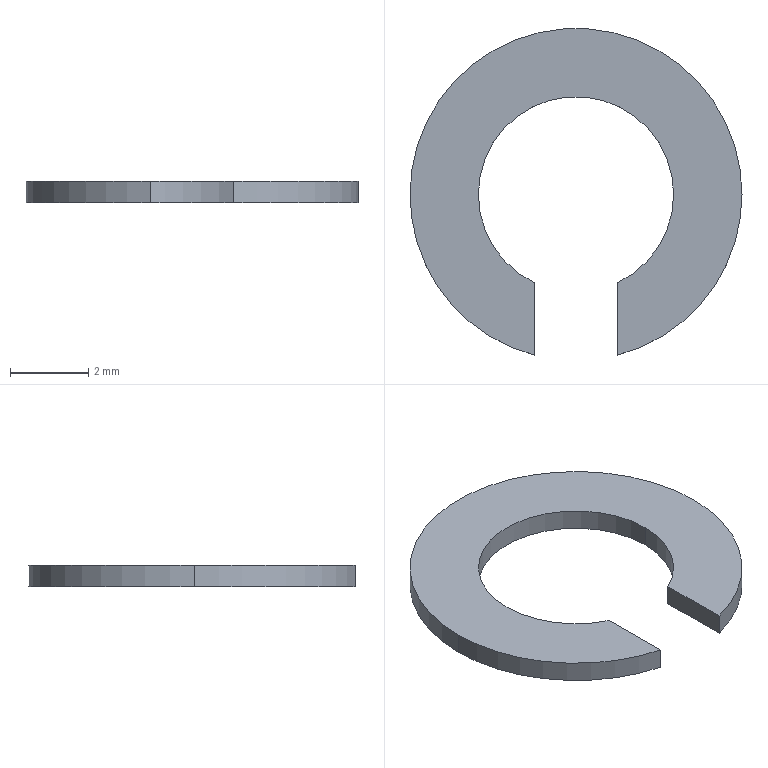Part | STEP file | 0245_Z_041_HCBST5-16_3 | 1 solid | 10 faces | box 8.5 x 8.364 x 0.54 mm | volume 17.989 mm3 | cylinder 6 | plane 4 | commonest cylinder face diameters 5 x3 8.5 x3
STEP:
#1=CARTESIAN_POINT('',(0.,0.,0.));
#2=DIRECTION('',(0.,0.,1.));
#3=DIRECTION('',(1.,0.,0.));
#4=AXIS2_PLACEMENT_3D('',#1,#2,#3);
#5=CARTESIAN_POINT('',(1.065,-2.262,0.54));
#6=VERTEX_POINT('',#5);
#7=CARTESIAN_POINT('',(1.065,-2.262,0.));
#8=VERTEX_POINT('',#7);
#9=CARTESIAN_POINT('',(1.065,-2.262,0.54));
#10=DIRECTION('',(0.,0.,-1.));
#11=VECTOR('',#10,1.);
#12=LINE('',#9,#11);
#13=CARTESIAN_POINT('',(0.,0.,0.54));
#14=DIRECTION('',(0.,0.,-1.));
#15=DIRECTION('',(-1.,0.,0.));
#16=AXIS2_PLACEMENT_3D('',#13,#14,#15);
#17=CYLINDRICAL_SURFACE('',#16,2.5);
#18=CARTESIAN_POINT('',(4.272,0.));
#19=DIRECTION('',(0.,1.));
#20=VECTOR('',#19,1.);
#21=LINE('',#18,#20);
#22=(GEOMETRIC_REPRESENTATION_CONTEXT(2)PARAMETRIC_REPRESENTATION_CONTEXT()REPRESENTATION_CONTEXT('',''));
#23=DEFINITIONAL_REPRESENTATION('',(#21),#22);
#24=PCURVE('',#17,#23);
#25=CARTESIAN_POINT('',(1.065,-2.262,0.54));
#26=DIRECTION('',(1.,0.,0.));
#27=DIRECTION('',(0.,1.,0.));
#28=AXIS2_PLACEMENT_3D('',#25,#26,#27);
#29=PLANE('',#28);
#30=CARTESIAN_POINT('',(0.,0.));
#31=DIRECTION('',(0.,-1.));
#32=VECTOR('',#31,1.);
#33=LINE('',#30,#32);
#34=(GEOMETRIC_REPRESENTATION_CONTEXT(2)PARAMETRIC_REPRESENTATION_CONTEXT()REPRESENTATION_CONTEXT('',''));
#35=DEFINITIONAL_REPRESENTATION('',(#33),#34);
#36=PCURVE('',#29,#35);
#37=SURFACE_CURVE('',#12,(#24,#36),.PCURVE_S1.);
#38=EDGE_CURVE('',#6,#8,#37,.T.);
#39=ORIENTED_EDGE('',*,*,#38,.T.);
#40=CARTESIAN_POINT('',(2.5,0.,0.));
#41=VERTEX_POINT('',#40);
#42=CARTESIAN_POINT('',(0.,0.,0.));
#43=DIRECTION('',(0.,0.,-1.));
#44=DIRECTION('',(1.,0.,0.));
#45=AXIS2_PLACEMENT_3D('',#42,#43,#44);
#46=CIRCLE('',#45,2.5);
#47=CARTESIAN_POINT('',(3.142,0.54));
#48=DIRECTION('',(1.,0.));
#49=VECTOR('',#48,1.);
#50=LINE('',#47,#49);
#51=(GEOMETRIC_REPRESENTATION_CONTEXT(2)PARAMETRIC_REPRESENTATION_CONTEXT()REPRESENTATION_CONTEXT('',''));
#52=DEFINITIONAL_REPRESENTATION('',(#50),#51);
#53=PCURVE('',#17,#52);
#54=CARTESIAN_POINT('',(0.,0.,0.));
#55=DIRECTION('',(0.,0.,1.));
#56=DIRECTION('',(1.,0.,0.));
#57=AXIS2_PLACEMENT_3D('',#54,#55,#56);
#58=PLANE('',#57);
#59=CARTESIAN_POINT('',(2.5,0.));
#60=CARTESIAN_POINT('',(2.5,-4.33));
#61=CARTESIAN_POINT('',(-1.25,-2.165));
#62=CARTESIAN_POINT('',(-5.,0.));
#63=CARTESIAN_POINT('',(-1.25,2.165));
#64=CARTESIAN_POINT('',(2.5,4.33));
#65=CARTESIAN_POINT('',(2.5,0.));
#66=(BOUNDED_CURVE()B_SPLINE_CURVE(2,(#59,#60,#61,#62,#63,#64,#65),.UNSPECIFIED.,.T.,.F.)B_SPLINE_CURVE_WITH_KNOTS((1,2,2,2,2,1),(-2.094,0.,2.094,4.189,6.283,8.378),.UNSPECIFIED.)CURVE()GEOMETRIC_REPRESENTATION_ITEM()RATIONAL_B_SPLINE_CURVE((1.,0.5,1.,0.5,1.,0.5,1.))REPRESENTATION_ITEM(''));
#67=(GEOMETRIC_REPRESENTATION_CONTEXT(2)PARAMETRIC_REPRESENTATION_CONTEXT()REPRESENTATION_CONTEXT('',''));
#68=DEFINITIONAL_REPRESENTATION('',(#66),#67);
#69=PCURVE('',#58,#68);
#70=SURFACE_CURVE('',#46,(#53,#69),.PCURVE_S1.);
#71=EDGE_CURVE('',#41,#8,#70,.T.);
#72=ORIENTED_EDGE('',*,*,#71,.F.);
#73=CARTESIAN_POINT('',(2.5,0.,0.54));
#74=VERTEX_POINT('',#73);
#75=CARTESIAN_POINT('',(2.5,0.,0.54));
#76=DIRECTION('',(0.,0.,-1.));
#77=VECTOR('',#76,1.);
#78=LINE('',#75,#77);
#79=CARTESIAN_POINT('',(3.142,0.));
#80=DIRECTION('',(0.,1.));
#81=VECTOR('',#80,1.);
#82=LINE('',#79,#81);
#83=(GEOMETRIC_REPRESENTATION_CONTEXT(2)PARAMETRIC_REPRESENTATION_CONTEXT()REPRESENTATION_CONTEXT('',''));
#84=DEFINITIONAL_REPRESENTATION('',(#82),#83);
#85=PCURVE('',#17,#84);
#86=CARTESIAN_POINT('',(0.,0.,0.54));
#87=DIRECTION('',(0.,0.,-1.));
#88=DIRECTION('',(-1.,0.,0.));
#89=AXIS2_PLACEMENT_3D('',#86,#87,#88);
#90=CYLINDRICAL_SURFACE('',#89,2.5);
#91=CARTESIAN_POINT('',(3.142,0.));
#92=DIRECTION('',(0.,1.));
#93=VECTOR('',#92,1.);
#94=LINE('',#91,#93);
#95=(GEOMETRIC_REPRESENTATION_CONTEXT(2)PARAMETRIC_REPRESENTATION_CONTEXT()REPRESENTATION_CONTEXT('',''));
#96=DEFINITIONAL_REPRESENTATION('',(#94),#95);
#97=PCURVE('',#90,#96);
#98=SURFACE_CURVE('',#78,(#85,#97),.PCURVE_S1.);
#99=EDGE_CURVE('',#74,#41,#98,.T.);
#100=ORIENTED_EDGE('',*,*,#99,.F.);
#101=CARTESIAN_POINT('',(0.,0.,0.54));
#102=DIRECTION('',(0.,0.,-1.));
#103=DIRECTION('',(1.,0.,0.));
#104=AXIS2_PLACEMENT_3D('',#101,#102,#103);
#105=CIRCLE('',#104,2.5);
#106=CARTESIAN_POINT('',(3.142,0.));
#107=DIRECTION('',(1.,0.));
#108=VECTOR('',#107,1.);
#109=LINE('',#106,#108);
#110=(GEOMETRIC_REPRESENTATION_CONTEXT(2)PARAMETRIC_REPRESENTATION_CONTEXT()REPRESENTATION_CONTEXT('',''));
#111=DEFINITIONAL_REPRESENTATION('',(#109),#110);
#112=PCURVE('',#17,#111);
#113=CARTESIAN_POINT('',(0.,0.,0.54));
#114=DIRECTION('',(0.,0.,1.));
#115=DIRECTION('',(1.,0.,0.));
#116=AXIS2_PLACEMENT_3D('',#113,#114,#115);
#117=PLANE('',#116);
#118=CARTESIAN_POINT('',(2.5,0.));
#119=CARTESIAN_POINT('',(2.5,-4.33));
#120=CARTESIAN_POINT('',(-1.25,-2.165));
#121=CARTESIAN_POINT('',(-5.,0.));
#122=CARTESIAN_POINT('',(-1.25,2.165));
#123=CARTESIAN_POINT('',(2.5,4.33));
#124=CARTESIAN_POINT('',(2.5,0.));
#125=(BOUNDED_CURVE()B_SPLINE_CURVE(2,(#118,#119,#120,#121,#122,#123,#124),.UNSPECIFIED.,.T.,.F.)B_SPLINE_CURVE_WITH_KNOTS((1,2,2,2,2,1),(-2.094,0.,2.094,4.189,6.283,8.378),.UNSPECIFIED.)CURVE()GEOMETRIC_REPRESENTATION_ITEM()RATIONAL_B_SPLINE_CURVE((1.,0.5,1.,0.5,1.,0.5,1.))REPRESENTATION_ITEM(''));
#126=(GEOMETRIC_REPRESENTATION_CONTEXT(2)PARAMETRIC_REPRESENTATION_CONTEXT()REPRESENTATION_CONTEXT('',''));
#127=DEFINITIONAL_REPRESENTATION('',(#125),#126);
#128=PCURVE('',#117,#127);
#129=SURFACE_CURVE('',#105,(#112,#128),.PCURVE_S1.);
#130=EDGE_CURVE('',#74,#6,#129,.T.);
#131=ORIENTED_EDGE('',*,*,#130,.T.);
#132=EDGE_LOOP('',(#39,#72,#100,#131));
#133=FACE_BOUND('',#132,.F.);
#134=ADVANCED_FACE('',(#133),#17,.F.);
#135=CARTESIAN_POINT('',(-2.5,0.,0.));
#136=VERTEX_POINT('',#135);
#137=CARTESIAN_POINT('',(0.,0.,0.));
#138=DIRECTION('',(0.,0.,-1.));
#139=DIRECTION('',(1.,0.,0.));
#140=AXIS2_PLACEMENT_3D('',#137,#138,#139);
#141=CIRCLE('',#140,2.5);
#142=CARTESIAN_POINT('',(-3.142,0.54));
#143=DIRECTION('',(1.,0.));
#144=VECTOR('',#143,1.);
#145=LINE('',#142,#144);
#146=(GEOMETRIC_REPRESENTATION_CONTEXT(2)PARAMETRIC_REPRESENTATION_CONTEXT()REPRESENTATION_CONTEXT('',''));
#147=DEFINITIONAL_REPRESENTATION('',(#145),#146);
#148=PCURVE('',#90,#147);
#149=CARTESIAN_POINT('',(2.5,0.));
#150=CARTESIAN_POINT('',(2.5,-4.33));
#151=CARTESIAN_POINT('',(-1.25,-2.165));
#152=CARTESIAN_POINT('',(-5.,0.));
#153=CARTESIAN_POINT('',(-1.25,2.165));
#154=CARTESIAN_POINT('',(2.5,4.33));
#155=CARTESIAN_POINT('',(2.5,0.));
#156=(BOUNDED_CURVE()B_SPLINE_CURVE(2,(#149,#150,#151,#152,#153,#154,#155),.UNSPECIFIED.,.T.,.F.)B_SPLINE_CURVE_WITH_KNOTS((1,2,2,2,2,1),(-2.094,0.,2.094,4.189,6.283,8.378),.UNSPECIFIED.)CURVE()GEOMETRIC_REPRESENTATION_ITEM()RATIONAL_B_SPLINE_CURVE((1.,0.5,1.,0.5,1.,0.5,1.))REPRESENTATION_ITEM(''));
#157=(GEOMETRIC_REPRESENTATION_CONTEXT(2)PARAMETRIC_REPRESENTATION_CONTEXT()REPRESENTATION_CONTEXT('',''));
#158=DEFINITIONAL_REPRESENTATION('',(#156),#157);
#159=PCURVE('',#58,#158);
#160=SURFACE_CURVE('',#141,(#148,#159),.PCURVE_S1.);
#161=EDGE_CURVE('',#136,#41,#160,.T.);
#162=ORIENTED_EDGE('',*,*,#161,.F.);
#163=CARTESIAN_POINT('',(-2.5,0.,0.54));
#164=VERTEX_POINT('',#163);
#165=CARTESIAN_POINT('',(-2.5,0.,0.54));
#166=DIRECTION('',(0.,0.,-1.));
#167=VECTOR('',#166,1.);
#168=LINE('',#165,#167);
#169=CARTESIAN_POINT('',(0.,0.));
#170=DIRECTION('',(0.,1.));
#171=VECTOR('',#170,1.);
#172=LINE('',#169,#171);
#173=(GEOMETRIC_REPRESENTATION_CONTEXT(2)PARAMETRIC_REPRESENTATION_CONTEXT()REPRESENTATION_CONTEXT('',''));
#174=DEFINITIONAL_REPRESENTATION('',(#172),#173);
#175=PCURVE('',#90,#174);
#176=CARTESIAN_POINT('',(0.,0.,0.54));
#177=DIRECTION('',(0.,0.,-1.));
#178=DIRECTION('',(-1.,0.,0.));
#179=AXIS2_PLACEMENT_3D('',#176,#177,#178);
#180=CYLINDRICAL_SURFACE('',#179,2.5);
#181=CARTESIAN_POINT('',(6.283,0.));
#182=DIRECTION('',(0.,1.));
#183=VECTOR('',#182,1.);
#184=LINE('',#181,#183);
#185=(GEOMETRIC_REPRESENTATION_CONTEXT(2)PARAMETRIC_REPRESENTATION_CONTEXT()REPRESENTATION_CONTEXT('',''));
#186=DEFINITIONAL_REPRESENTATION('',(#184),#185);
#187=PCURVE('',#180,#186);
#188=SURFACE_CURVE('',#168,(#175,#187),.PCURVE_S1.);
#189=EDGE_CURVE('',#164,#136,#188,.T.);
#190=ORIENTED_EDGE('',*,*,#189,.F.);
#191=CARTESIAN_POINT('',(0.,0.,0.54));
#192=DIRECTION('',(0.,0.,-1.));
#193=DIRECTION('',(1.,0.,0.));
#194=AXIS2_PLACEMENT_3D('',#191,#192,#193);
#195=CIRCLE('',#194,2.5);
#196=CARTESIAN_POINT('',(-3.142,0.));
#197=DIRECTION('',(1.,0.));
#198=VECTOR('',#197,1.);
#199=LINE('',#196,#198);
#200=(GEOMETRIC_REPRESENTATION_CONTEXT(2)PARAMETRIC_REPRESENTATION_CONTEXT()REPRESENTATION_CONTEXT('',''));
#201=DEFINITIONAL_REPRESENTATION('',(#199),#200);
#202=PCURVE('',#90,#201);
#203=CARTESIAN_POINT('',(2.5,0.));
#204=CARTESIAN_POINT('',(2.5,-4.33));
#205=CARTESIAN_POINT('',(-1.25,-2.165));
#206=CARTESIAN_POINT('',(-5.,0.));
#207=CARTESIAN_POINT('',(-1.25,2.165));
#208=CARTESIAN_POINT('',(2.5,4.33));
#209=CARTESIAN_POINT('',(2.5,0.));
#210=(BOUNDED_CURVE()B_SPLINE_CURVE(2,(#203,#204,#205,#206,#207,#208,#209),.UNSPECIFIED.,.T.,.F.)B_SPLINE_CURVE_WITH_KNOTS((1,2,2,2,2,1),(-2.094,0.,2.094,4.189,6.283,8.378),.UNSPECIFIED.)CURVE()GEOMETRIC_REPRESENTATION_ITEM()RATIONAL_B_SPLINE_CURVE((1.,0.5,1.,0.5,1.,0.5,1.))REPRESENTATION_ITEM(''));
#211=(GEOMETRIC_REPRESENTATION_CONTEXT(2)PARAMETRIC_REPRESENTATION_CONTEXT()REPRESENTATION_CONTEXT('',''));
#212=DEFINITIONAL_REPRESENTATION('',(#210),#211);
#213=PCURVE('',#117,#212);
#214=SURFACE_CURVE('',#195,(#202,#213),.PCURVE_S1.);
#215=EDGE_CURVE('',#164,#74,#214,.T.);
#216=ORIENTED_EDGE('',*,*,#215,.T.);
#217=ORIENTED_EDGE('',*,*,#99,.T.);
#218=EDGE_LOOP('',(#162,#190,#216,#217));
#219=FACE_BOUND('',#218,.F.);
#220=ADVANCED_FACE('',(#219),#90,.F.);
#221=CARTESIAN_POINT('',(4.25,0.,0.54));
#222=VERTEX_POINT('',#221);
#223=CARTESIAN_POINT('',(-4.25,0.,0.54));
#224=VERTEX_POINT('',#223);
#225=CARTESIAN_POINT('',(0.,0.,0.54));
#226=DIRECTION('',(0.,0.,1.));
#227=DIRECTION('',(1.,0.,0.));
#228=AXIS2_PLACEMENT_3D('',#225,#226,#227);
#229=CIRCLE('',#228,4.25);
#230=CARTESIAN_POINT('',(0.,0.,0.54));
#231=DIRECTION('',(0.,0.,-1.));
#232=DIRECTION('',(-1.,0.,0.));
#233=AXIS2_PLACEMENT_3D('',#230,#231,#232);
#234=CYLINDRICAL_SURFACE('',#233,4.25);
#235=CARTESIAN_POINT('',(3.142,0.));
#236=DIRECTION('',(-1.,0.));
#237=VECTOR('',#236,1.);
#238=LINE('',#235,#237);
#239=(GEOMETRIC_REPRESENTATION_CONTEXT(2)PARAMETRIC_REPRESENTATION_CONTEXT()REPRESENTATION_CONTEXT('',''));
#240=DEFINITIONAL_REPRESENTATION('',(#238),#239);
#241=PCURVE('',#234,#240);
#242=CARTESIAN_POINT('',(0.,0.));
#243=DIRECTION('',(1.,0.));
#244=AXIS2_PLACEMENT_2D('',#242,#243);
#245=CIRCLE('',#244,4.25);
#246=(GEOMETRIC_REPRESENTATION_CONTEXT(2)PARAMETRIC_REPRESENTATION_CONTEXT()REPRESENTATION_CONTEXT('',''));
#247=DEFINITIONAL_REPRESENTATION('',(#245),#246);
#248=PCURVE('',#117,#247);
#249=SURFACE_CURVE('',#229,(#241,#248),.PCURVE_S1.);
#250=EDGE_CURVE('',#222,#224,#249,.T.);
#251=ORIENTED_EDGE('',*,*,#250,.F.);
#252=CARTESIAN_POINT('',(4.25,0.,0.));
#253=VERTEX_POINT('',#252);
#254=CARTESIAN_POINT('',(4.25,0.,0.54));
#255=DIRECTION('',(0.,0.,-1.));
#256=VECTOR('',#255,1.);
#257=LINE('',#254,#256);
#258=CARTESIAN_POINT('',(3.142,0.));
#259=DIRECTION('',(0.,1.));
#260=VECTOR('',#259,1.);
#261=LINE('',#258,#260);
#262=(GEOMETRIC_REPRESENTATION_CONTEXT(2)PARAMETRIC_REPRESENTATION_CONTEXT()REPRESENTATION_CONTEXT('',''));
#263=DEFINITIONAL_REPRESENTATION('',(#261),#262);
#264=PCURVE('',#234,#263);
#265=CARTESIAN_POINT('',(0.,0.,0.54));
#266=DIRECTION('',(0.,0.,-1.));
#267=DIRECTION('',(-1.,0.,0.));
#268=AXIS2_PLACEMENT_3D('',#265,#266,#267);
#269=CYLINDRICAL_SURFACE('',#268,4.25);
#270=CARTESIAN_POINT('',(3.142,0.));
#271=DIRECTION('',(0.,1.));
#272=VECTOR('',#271,1.);
#273=LINE('',#270,#272);
#274=(GEOMETRIC_REPRESENTATION_CONTEXT(2)PARAMETRIC_REPRESENTATION_CONTEXT()REPRESENTATION_CONTEXT('',''));
#275=DEFINITIONAL_REPRESENTATION('',(#273),#274);
#276=PCURVE('',#269,#275);
#277=SURFACE_CURVE('',#257,(#264,#276),.PCURVE_S1.);
#278=EDGE_CURVE('',#222,#253,#277,.T.);
#279=ORIENTED_EDGE('',*,*,#278,.T.);
#280=CARTESIAN_POINT('',(-4.25,0.,0.));
#281=VERTEX_POINT('',#280);
#282=CARTESIAN_POINT('',(0.,0.,0.));
#283=DIRECTION('',(0.,0.,1.));
#284=DIRECTION('',(1.,0.,0.));
#285=AXIS2_PLACEMENT_3D('',#282,#283,#284);
#286=CIRCLE('',#285,4.25);
#287=CARTESIAN_POINT('',(3.142,0.54));
#288=DIRECTION('',(-1.,0.));
#289=VECTOR('',#288,1.);
#290=LINE('',#287,#289);
#291=(GEOMETRIC_REPRESENTATION_CONTEXT(2)PARAMETRIC_REPRESENTATION_CONTEXT()REPRESENTATION_CONTEXT('',''));
#292=DEFINITIONAL_REPRESENTATION('',(#290),#291);
#293=PCURVE('',#234,#292);
#294=CARTESIAN_POINT('',(0.,0.));
#295=DIRECTION('',(1.,0.));
#296=AXIS2_PLACEMENT_2D('',#294,#295);
#297=CIRCLE('',#296,4.25);
#298=(GEOMETRIC_REPRESENTATION_CONTEXT(2)PARAMETRIC_REPRESENTATION_CONTEXT()REPRESENTATION_CONTEXT('',''));
#299=DEFINITIONAL_REPRESENTATION('',(#297),#298);
#300=PCURVE('',#58,#299);
#301=SURFACE_CURVE('',#286,(#293,#300),.PCURVE_S1.);
#302=EDGE_CURVE('',#253,#281,#301,.T.);
#303=ORIENTED_EDGE('',*,*,#302,.T.);
#304=CARTESIAN_POINT('',(-4.25,0.,0.54));
#305=DIRECTION('',(0.,0.,-1.));
#306=VECTOR('',#305,1.);
#307=LINE('',#304,#306);
#308=CARTESIAN_POINT('',(0.,0.));
#309=DIRECTION('',(0.,1.));
#310=VECTOR('',#309,1.);
#311=LINE('',#308,#310);
#312=(GEOMETRIC_REPRESENTATION_CONTEXT(2)PARAMETRIC_REPRESENTATION_CONTEXT()REPRESENTATION_CONTEXT('',''));
#313=DEFINITIONAL_REPRESENTATION('',(#311),#312);
#314=PCURVE('',#234,#313);
#315=CARTESIAN_POINT('',(0.,0.,0.54));
#316=DIRECTION('',(0.,0.,-1.));
#317=DIRECTION('',(-1.,0.,0.));
#318=AXIS2_PLACEMENT_3D('',#315,#316,#317);
#319=CYLINDRICAL_SURFACE('',#318,4.25);
#320=CARTESIAN_POINT('',(6.283,0.));
#321=DIRECTION('',(0.,1.));
#322=VECTOR('',#321,1.);
#323=LINE('',#320,#322);
#324=(GEOMETRIC_REPRESENTATION_CONTEXT(2)PARAMETRIC_REPRESENTATION_CONTEXT()REPRESENTATION_CONTEXT('',''));
#325=DEFINITIONAL_REPRESENTATION('',(#323),#324);
#326=PCURVE('',#319,#325);
#327=SURFACE_CURVE('',#307,(#314,#326),.PCURVE_S1.);
#328=EDGE_CURVE('',#224,#281,#327,.T.);
#329=ORIENTED_EDGE('',*,*,#328,.F.);
#330=EDGE_LOOP('',(#251,#279,#303,#329));
#331=FACE_BOUND('',#330,.T.);
#332=ADVANCED_FACE('',(#331),#234,.T.);
#333=CARTESIAN_POINT('',(-1.065,-4.114,0.54));
#334=VERTEX_POINT('',#333);
#335=CARTESIAN_POINT('',(0.,0.,0.54));
#336=DIRECTION('',(0.,0.,1.));
#337=DIRECTION('',(1.,0.,0.));
#338=AXIS2_PLACEMENT_3D('',#335,#336,#337);
#339=CIRCLE('',#338,4.25);
#340=CARTESIAN_POINT('',(9.425,0.));
#341=DIRECTION('',(-1.,0.));
#342=VECTOR('',#341,1.);
#343=LINE('',#340,#342);
#344=(GEOMETRIC_REPRESENTATION_CONTEXT(2)PARAMETRIC_REPRESENTATION_CONTEXT()REPRESENTATION_CONTEXT('',''));
#345=DEFINITIONAL_REPRESENTATION('',(#343),#344);
#346=PCURVE('',#319,#345);
#347=CARTESIAN_POINT('',(0.,0.));
#348=DIRECTION('',(1.,0.));
#349=AXIS2_PLACEMENT_2D('',#347,#348);
#350=CIRCLE('',#349,4.25);
#351=(GEOMETRIC_REPRESENTATION_CONTEXT(2)PARAMETRIC_REPRESENTATION_CONTEXT()REPRESENTATION_CONTEXT('',''));
#352=DEFINITIONAL_REPRESENTATION('',(#350),#351);
#353=PCURVE('',#117,#352);
#354=SURFACE_CURVE('',#339,(#346,#353),.PCURVE_S1.);
#355=EDGE_CURVE('',#224,#334,#354,.T.);
#356=ORIENTED_EDGE('',*,*,#355,.F.);
#357=ORIENTED_EDGE('',*,*,#328,.T.);
#358=CARTESIAN_POINT('',(-1.065,-4.114,0.));
#359=VERTEX_POINT('',#358);
#360=CARTESIAN_POINT('',(0.,0.,0.));
#361=DIRECTION('',(0.,0.,1.));
#362=DIRECTION('',(1.,0.,0.));
#363=AXIS2_PLACEMENT_3D('',#360,#361,#362);
#364=CIRCLE('',#363,4.25);
#365=CARTESIAN_POINT('',(9.425,0.54));
#366=DIRECTION('',(-1.,0.));
#367=VECTOR('',#366,1.);
#368=LINE('',#365,#367);
#369=(GEOMETRIC_REPRESENTATION_CONTEXT(2)PARAMETRIC_REPRESENTATION_CONTEXT()REPRESENTATION_CONTEXT('',''));
#370=DEFINITIONAL_REPRESENTATION('',(#368),#369);
#371=PCURVE('',#319,#370);
#372=CARTESIAN_POINT('',(0.,0.));
#373=DIRECTION('',(1.,0.));
#374=AXIS2_PLACEMENT_2D('',#372,#373);
#375=CIRCLE('',#374,4.25);
#376=(GEOMETRIC_REPRESENTATION_CONTEXT(2)PARAMETRIC_REPRESENTATION_CONTEXT()REPRESENTATION_CONTEXT('',''));
#377=DEFINITIONAL_REPRESENTATION('',(#375),#376);
#378=PCURVE('',#58,#377);
#379=SURFACE_CURVE('',#364,(#371,#378),.PCURVE_S1.);
#380=EDGE_CURVE('',#281,#359,#379,.T.);
#381=ORIENTED_EDGE('',*,*,#380,.T.);
#382=CARTESIAN_POINT('',(-1.065,-4.114,0.54));
#383=DIRECTION('',(0.,0.,-1.));
#384=VECTOR('',#383,1.);
#385=LINE('',#382,#384);
#386=CARTESIAN_POINT('',(4.966,0.));
#387=DIRECTION('',(0.,1.));
#388=VECTOR('',#387,1.);
#389=LINE('',#386,#388);
#390=(GEOMETRIC_REPRESENTATION_CONTEXT(2)PARAMETRIC_REPRESENTATION_CONTEXT()REPRESENTATION_CONTEXT('',''));
#391=DEFINITIONAL_REPRESENTATION('',(#389),#390);
#392=PCURVE('',#319,#391);
#393=CARTESIAN_POINT('',(-1.065,-2.262,0.54));
#394=DIRECTION('',(-1.,0.,0.));
#395=DIRECTION('',(0.,-1.,0.));
#396=AXIS2_PLACEMENT_3D('',#393,#394,#395);
#397=PLANE('',#396);
#398=CARTESIAN_POINT('',(1.853,0.));
#399=DIRECTION('',(0.,-1.));
#400=VECTOR('',#399,1.);
#401=LINE('',#398,#400);
#402=(GEOMETRIC_REPRESENTATION_CONTEXT(2)PARAMETRIC_REPRESENTATION_CONTEXT()REPRESENTATION_CONTEXT('',''));
#403=DEFINITIONAL_REPRESENTATION('',(#401),#402);
#404=PCURVE('',#397,#403);
#405=SURFACE_CURVE('',#385,(#392,#404),.PCURVE_S1.);
#406=EDGE_CURVE('',#334,#359,#405,.T.);
#407=ORIENTED_EDGE('',*,*,#406,.F.);
#408=EDGE_LOOP('',(#356,#357,#381,#407));
#409=FACE_BOUND('',#408,.T.);
#410=ADVANCED_FACE('',(#409),#319,.T.);
#411=ORIENTED_EDGE('',*,*,#278,.F.);
#412=CARTESIAN_POINT('',(1.065,-4.114,0.54));
#413=VERTEX_POINT('',#412);
#414=CARTESIAN_POINT('',(0.,0.,0.54));
#415=DIRECTION('',(0.,0.,1.));
#416=DIRECTION('',(1.,0.,0.));
#417=AXIS2_PLACEMENT_3D('',#414,#415,#416);
#418=CIRCLE('',#417,4.25);
#419=CARTESIAN_POINT('',(9.425,0.));
#420=DIRECTION('',(-1.,0.));
#421=VECTOR('',#420,1.);
#422=LINE('',#419,#421);
#423=(GEOMETRIC_REPRESENTATION_CONTEXT(2)PARAMETRIC_REPRESENTATION_CONTEXT()REPRESENTATION_CONTEXT('',''));
#424=DEFINITIONAL_REPRESENTATION('',(#422),#423);
#425=PCURVE('',#269,#424);
#426=CARTESIAN_POINT('',(0.,0.));
#427=DIRECTION('',(1.,0.));
#428=AXIS2_PLACEMENT_2D('',#426,#427);
#429=CIRCLE('',#428,4.25);
#430=(GEOMETRIC_REPRESENTATION_CONTEXT(2)PARAMETRIC_REPRESENTATION_CONTEXT()REPRESENTATION_CONTEXT('',''));
#431=DEFINITIONAL_REPRESENTATION('',(#429),#430);
#432=PCURVE('',#117,#431);
#433=SURFACE_CURVE('',#418,(#425,#432),.PCURVE_S1.);
#434=EDGE_CURVE('',#413,#222,#433,.T.);
#435=ORIENTED_EDGE('',*,*,#434,.F.);
#436=CARTESIAN_POINT('',(1.065,-4.114,0.));
#437=VERTEX_POINT('',#436);
#438=CARTESIAN_POINT('',(1.065,-4.114,0.54));
#439=DIRECTION('',(0.,0.,-1.));
#440=VECTOR('',#439,1.);
#441=LINE('',#438,#440);
#442=CARTESIAN_POINT('',(4.459,0.));
#443=DIRECTION('',(0.,1.));
#444=VECTOR('',#443,1.);
#445=LINE('',#442,#444);
#446=(GEOMETRIC_REPRESENTATION_CONTEXT(2)PARAMETRIC_REPRESENTATION_CONTEXT()REPRESENTATION_CONTEXT('',''));
#447=DEFINITIONAL_REPRESENTATION('',(#445),#446);
#448=PCURVE('',#269,#447);
#449=CARTESIAN_POINT('',(-1.853,0.));
#450=DIRECTION('',(0.,-1.));
#451=VECTOR('',#450,1.);
#452=LINE('',#449,#451);
#453=(GEOMETRIC_REPRESENTATION_CONTEXT(2)PARAMETRIC_REPRESENTATION_CONTEXT()REPRESENTATION_CONTEXT('',''));
#454=DEFINITIONAL_REPRESENTATION('',(#452),#453);
#455=PCURVE('',#29,#454);
#456=SURFACE_CURVE('',#441,(#448,#455),.PCURVE_S1.);
#457=EDGE_CURVE('',#413,#437,#456,.T.);
#458=ORIENTED_EDGE('',*,*,#457,.T.);
#459=CARTESIAN_POINT('',(0.,0.,0.));
#460=DIRECTION('',(0.,0.,1.));
#461=DIRECTION('',(1.,0.,0.));
#462=AXIS2_PLACEMENT_3D('',#459,#460,#461);
#463=CIRCLE('',#462,4.25);
#464=CARTESIAN_POINT('',(9.425,0.54));
#465=DIRECTION('',(-1.,0.));
#466=VECTOR('',#465,1.);
#467=LINE('',#464,#466);
#468=(GEOMETRIC_REPRESENTATION_CONTEXT(2)PARAMETRIC_REPRESENTATION_CONTEXT()REPRESENTATION_CONTEXT('',''));
#469=DEFINITIONAL_REPRESENTATION('',(#467),#468);
#470=PCURVE('',#269,#469);
#471=CARTESIAN_POINT('',(0.,0.));
#472=DIRECTION('',(1.,0.));
#473=AXIS2_PLACEMENT_2D('',#471,#472);
#474=CIRCLE('',#473,4.25);
#475=(GEOMETRIC_REPRESENTATION_CONTEXT(2)PARAMETRIC_REPRESENTATION_CONTEXT()REPRESENTATION_CONTEXT('',''));
#476=DEFINITIONAL_REPRESENTATION('',(#474),#475);
#477=PCURVE('',#58,#476);
#478=SURFACE_CURVE('',#463,(#470,#477),.PCURVE_S1.);
#479=EDGE_CURVE('',#437,#253,#478,.T.);
#480=ORIENTED_EDGE('',*,*,#479,.T.);
#481=EDGE_LOOP('',(#411,#435,#458,#480));
#482=FACE_BOUND('',#481,.T.);
#483=ADVANCED_FACE('',(#482),#269,.T.);
#484=CARTESIAN_POINT('',(-1.065,-2.262,0.));
#485=VERTEX_POINT('',#484);
#486=CARTESIAN_POINT('',(-1.065,-2.262,0.));
#487=DIRECTION('',(0.,1.,0.));
#488=VECTOR('',#487,1.);
#489=LINE('',#486,#488);
#490=CARTESIAN_POINT('',(0.,-0.54));
#491=DIRECTION('',(-1.,0.));
#492=VECTOR('',#491,1.);
#493=LINE('',#490,#492);
#494=(GEOMETRIC_REPRESENTATION_CONTEXT(2)PARAMETRIC_REPRESENTATION_CONTEXT()REPRESENTATION_CONTEXT('',''));
#495=DEFINITIONAL_REPRESENTATION('',(#493),#494);
#496=PCURVE('',#397,#495);
#497=CARTESIAN_POINT('',(-1.065,-2.262));
#498=DIRECTION('',(0.,1.));
#499=VECTOR('',#498,1.);
#500=LINE('',#497,#499);
#501=(GEOMETRIC_REPRESENTATION_CONTEXT(2)PARAMETRIC_REPRESENTATION_CONTEXT()REPRESENTATION_CONTEXT('',''));
#502=DEFINITIONAL_REPRESENTATION('',(#500),#501);
#503=PCURVE('',#58,#502);
#504=SURFACE_CURVE('',#489,(#496,#503),.PCURVE_S1.);
#505=EDGE_CURVE('',#359,#485,#504,.T.);
#506=ORIENTED_EDGE('',*,*,#505,.T.);
#507=CARTESIAN_POINT('',(-1.065,-2.262,0.54));
#508=VERTEX_POINT('',#507);
#509=CARTESIAN_POINT('',(-1.065,-2.262,0.54));
#510=DIRECTION('',(0.,0.,-1.));
#511=VECTOR('',#510,1.);
#512=LINE('',#509,#511);
#513=CARTESIAN_POINT('',(0.,0.));
#514=DIRECTION('',(0.,-1.));
#515=VECTOR('',#514,1.);
#516=LINE('',#513,#515);
#517=(GEOMETRIC_REPRESENTATION_CONTEXT(2)PARAMETRIC_REPRESENTATION_CONTEXT()REPRESENTATION_CONTEXT('',''));
#518=DEFINITIONAL_REPRESENTATION('',(#516),#517);
#519=PCURVE('',#397,#518);
#520=CARTESIAN_POINT('',(5.152,0.));
#521=DIRECTION('',(0.,1.));
#522=VECTOR('',#521,1.);
#523=LINE('',#520,#522);
#524=(GEOMETRIC_REPRESENTATION_CONTEXT(2)PARAMETRIC_REPRESENTATION_CONTEXT()REPRESENTATION_CONTEXT('',''));
#525=DEFINITIONAL_REPRESENTATION('',(#523),#524);
#526=PCURVE('',#180,#525);
#527=SURFACE_CURVE('',#512,(#519,#526),.PCURVE_S1.);
#528=EDGE_CURVE('',#508,#485,#527,.T.);
#529=ORIENTED_EDGE('',*,*,#528,.F.);
#530=CARTESIAN_POINT('',(-1.065,-2.262,0.54));
#531=DIRECTION('',(0.,1.,0.));
#532=VECTOR('',#531,1.);
#533=LINE('',#530,#532);
#534=CARTESIAN_POINT('',(0.,0.));
#535=DIRECTION('',(-1.,0.));
#536=VECTOR('',#535,1.);
#537=LINE('',#534,#536);
#538=(GEOMETRIC_REPRESENTATION_CONTEXT(2)PARAMETRIC_REPRESENTATION_CONTEXT()REPRESENTATION_CONTEXT('',''));
#539=DEFINITIONAL_REPRESENTATION('',(#537),#538);
#540=PCURVE('',#397,#539);
#541=CARTESIAN_POINT('',(-1.065,-2.262));
#542=DIRECTION('',(0.,1.));
#543=VECTOR('',#542,1.);
#544=LINE('',#541,#543);
#545=(GEOMETRIC_REPRESENTATION_CONTEXT(2)PARAMETRIC_REPRESENTATION_CONTEXT()REPRESENTATION_CONTEXT('',''));
#546=DEFINITIONAL_REPRESENTATION('',(#544),#545);
#547=PCURVE('',#117,#546);
#548=SURFACE_CURVE('',#533,(#540,#547),.PCURVE_S1.);
#549=EDGE_CURVE('',#334,#508,#548,.T.);
#550=ORIENTED_EDGE('',*,*,#549,.F.);
#551=ORIENTED_EDGE('',*,*,#406,.T.);
#552=EDGE_LOOP('',(#506,#529,#550,#551));
#553=FACE_BOUND('',#552,.T.);
#554=ADVANCED_FACE('',(#553),#397,.F.);
#555=CARTESIAN_POINT('',(0.,0.,0.));
#556=DIRECTION('',(0.,0.,-1.));
#557=DIRECTION('',(1.,0.,0.));
#558=AXIS2_PLACEMENT_3D('',#555,#556,#557);
#559=CIRCLE('',#558,2.5);
#560=CARTESIAN_POINT('',(3.142,0.54));
#561=DIRECTION('',(1.,0.));
#562=VECTOR('',#561,1.);
#563=LINE('',#560,#562);
#564=(GEOMETRIC_REPRESENTATION_CONTEXT(2)PARAMETRIC_REPRESENTATION_CONTEXT()REPRESENTATION_CONTEXT('',''));
#565=DEFINITIONAL_REPRESENTATION('',(#563),#564);
#566=PCURVE('',#180,#565);
#567=CARTESIAN_POINT('',(2.5,0.));
#568=CARTESIAN_POINT('',(2.5,-4.33));
#569=CARTESIAN_POINT('',(-1.25,-2.165));
#570=CARTESIAN_POINT('',(-5.,0.));
#571=CARTESIAN_POINT('',(-1.25,2.165));
#572=CARTESIAN_POINT('',(2.5,4.33));
#573=CARTESIAN_POINT('',(2.5,0.));
#574=(BOUNDED_CURVE()B_SPLINE_CURVE(2,(#567,#568,#569,#570,#571,#572,#573),.UNSPECIFIED.,.T.,.F.)B_SPLINE_CURVE_WITH_KNOTS((1,2,2,2,2,1),(-2.094,0.,2.094,4.189,6.283,8.378),.UNSPECIFIED.)CURVE()GEOMETRIC_REPRESENTATION_ITEM()RATIONAL_B_SPLINE_CURVE((1.,0.5,1.,0.5,1.,0.5,1.))REPRESENTATION_ITEM(''));
#575=(GEOMETRIC_REPRESENTATION_CONTEXT(2)PARAMETRIC_REPRESENTATION_CONTEXT()REPRESENTATION_CONTEXT('',''));
#576=DEFINITIONAL_REPRESENTATION('',(#574),#575);
#577=PCURVE('',#58,#576);
#578=SURFACE_CURVE('',#559,(#566,#577),.PCURVE_S1.);
#579=EDGE_CURVE('',#485,#136,#578,.T.);
#580=ORIENTED_EDGE('',*,*,#579,.F.);
#581=ORIENTED_EDGE('',*,*,#528,.F.);
#582=CARTESIAN_POINT('',(0.,0.,0.54));
#583=DIRECTION('',(0.,0.,-1.));
#584=DIRECTION('',(1.,0.,0.));
#585=AXIS2_PLACEMENT_3D('',#582,#583,#584);
#586=CIRCLE('',#585,2.5);
#587=CARTESIAN_POINT('',(3.142,0.));
#588=DIRECTION('',(1.,0.));
#589=VECTOR('',#588,1.);
#590=LINE('',#587,#589);
#591=(GEOMETRIC_REPRESENTATION_CONTEXT(2)PARAMETRIC_REPRESENTATION_CONTEXT()REPRESENTATION_CONTEXT('',''));
#592=DEFINITIONAL_REPRESENTATION('',(#590),#591);
#593=PCURVE('',#180,#592);
#594=CARTESIAN_POINT('',(2.5,0.));
#595=CARTESIAN_POINT('',(2.5,-4.33));
#596=CARTESIAN_POINT('',(-1.25,-2.165));
#597=CARTESIAN_POINT('',(-5.,0.));
#598=CARTESIAN_POINT('',(-1.25,2.165));
#599=CARTESIAN_POINT('',(2.5,4.33));
#600=CARTESIAN_POINT('',(2.5,0.));
#601=(BOUNDED_CURVE()B_SPLINE_CURVE(2,(#594,#595,#596,#597,#598,#599,#600),.UNSPECIFIED.,.T.,.F.)B_SPLINE_CURVE_WITH_KNOTS((1,2,2,2,2,1),(-2.094,0.,2.094,4.189,6.283,8.378),.UNSPECIFIED.)CURVE()GEOMETRIC_REPRESENTATION_ITEM()RATIONAL_B_SPLINE_CURVE((1.,0.5,1.,0.5,1.,0.5,1.))REPRESENTATION_ITEM(''));
#602=(GEOMETRIC_REPRESENTATION_CONTEXT(2)PARAMETRIC_REPRESENTATION_CONTEXT()REPRESENTATION_CONTEXT('',''));
#603=DEFINITIONAL_REPRESENTATION('',(#601),#602);
#604=PCURVE('',#117,#603);
#605=SURFACE_CURVE('',#586,(#593,#604),.PCURVE_S1.);
#606=EDGE_CURVE('',#508,#164,#605,.T.);
#607=ORIENTED_EDGE('',*,*,#606,.T.);
#608=ORIENTED_EDGE('',*,*,#189,.T.);
#609=EDGE_LOOP('',(#580,#581,#607,#608));
#610=FACE_BOUND('',#609,.F.);
#611=ADVANCED_FACE('',(#610),#180,.F.);
#612=CARTESIAN_POINT('',(1.065,-2.262,0.));
#613=DIRECTION('',(0.,-1.,0.));
#614=VECTOR('',#613,1.);
#615=LINE('',#612,#614);
#616=CARTESIAN_POINT('',(0.,-0.54));
#617=DIRECTION('',(-1.,0.));
#618=VECTOR('',#617,1.);
#619=LINE('',#616,#618);
#620=(GEOMETRIC_REPRESENTATION_CONTEXT(2)PARAMETRIC_REPRESENTATION_CONTEXT()REPRESENTATION_CONTEXT('',''));
#621=DEFINITIONAL_REPRESENTATION('',(#619),#620);
#622=PCURVE('',#29,#621);
#623=CARTESIAN_POINT('',(1.065,-2.262));
#624=DIRECTION('',(0.,-1.));
#625=VECTOR('',#624,1.);
#626=LINE('',#623,#625);
#627=(GEOMETRIC_REPRESENTATION_CONTEXT(2)PARAMETRIC_REPRESENTATION_CONTEXT()REPRESENTATION_CONTEXT('',''));
#628=DEFINITIONAL_REPRESENTATION('',(#626),#627);
#629=PCURVE('',#58,#628);
#630=SURFACE_CURVE('',#615,(#622,#629),.PCURVE_S1.);
#631=EDGE_CURVE('',#8,#437,#630,.T.);
#632=ORIENTED_EDGE('',*,*,#631,.T.);
#633=ORIENTED_EDGE('',*,*,#457,.F.);
#634=CARTESIAN_POINT('',(1.065,-2.262,0.54));
#635=DIRECTION('',(0.,-1.,0.));
#636=VECTOR('',#635,1.);
#637=LINE('',#634,#636);
#638=CARTESIAN_POINT('',(0.,0.));
#639=DIRECTION('',(-1.,0.));
#640=VECTOR('',#639,1.);
#641=LINE('',#638,#640);
#642=(GEOMETRIC_REPRESENTATION_CONTEXT(2)PARAMETRIC_REPRESENTATION_CONTEXT()REPRESENTATION_CONTEXT('',''));
#643=DEFINITIONAL_REPRESENTATION('',(#641),#642);
#644=PCURVE('',#29,#643);
#645=CARTESIAN_POINT('',(1.065,-2.262));
#646=DIRECTION('',(0.,-1.));
#647=VECTOR('',#646,1.);
#648=LINE('',#645,#647);
#649=(GEOMETRIC_REPRESENTATION_CONTEXT(2)PARAMETRIC_REPRESENTATION_CONTEXT()REPRESENTATION_CONTEXT('',''));
#650=DEFINITIONAL_REPRESENTATION('',(#648),#649);
#651=PCURVE('',#117,#650);
#652=SURFACE_CURVE('',#637,(#644,#651),.PCURVE_S1.);
#653=EDGE_CURVE('',#6,#413,#652,.T.);
#654=ORIENTED_EDGE('',*,*,#653,.F.);
#655=ORIENTED_EDGE('',*,*,#38,.T.);
#656=EDGE_LOOP('',(#632,#633,#654,#655));
#657=FACE_BOUND('',#656,.T.);
#658=ADVANCED_FACE('',(#657),#29,.F.);
#659=ORIENTED_EDGE('',*,*,#434,.T.);
#660=ORIENTED_EDGE('',*,*,#250,.T.);
#661=ORIENTED_EDGE('',*,*,#355,.T.);
#662=ORIENTED_EDGE('',*,*,#549,.T.);
#663=ORIENTED_EDGE('',*,*,#606,.T.);
#664=ORIENTED_EDGE('',*,*,#215,.T.);
#665=ORIENTED_EDGE('',*,*,#130,.T.);
#666=ORIENTED_EDGE('',*,*,#653,.T.);
#667=EDGE_LOOP('',(#659,#660,#661,#662,#663,#664,#665,#666));
#668=FACE_BOUND('',#667,.T.);
#669=ADVANCED_FACE('',(#668),#117,.T.);
#670=ORIENTED_EDGE('',*,*,#479,.F.);
#671=ORIENTED_EDGE('',*,*,#631,.F.);
#672=ORIENTED_EDGE('',*,*,#71,.F.);
#673=ORIENTED_EDGE('',*,*,#161,.F.);
#674=ORIENTED_EDGE('',*,*,#579,.F.);
#675=ORIENTED_EDGE('',*,*,#505,.F.);
#676=ORIENTED_EDGE('',*,*,#380,.F.);
#677=ORIENTED_EDGE('',*,*,#302,.F.);
#678=EDGE_LOOP('',(#670,#671,#672,#673,#674,#675,#676,#677));
#679=FACE_BOUND('',#678,.T.);
#680=ADVANCED_FACE('',(#679),#58,.F.);
#681=CLOSED_SHELL('',(#134,#220,#332,#410,#483,#554,#611,#658,#669,#680));
#682=MANIFOLD_SOLID_BREP('',#681);
#683=(LENGTH_UNIT()NAMED_UNIT(*)SI_UNIT(.MILLI.,.METRE.));
#684=UNCERTAINTY_MEASURE_WITH_UNIT(LENGTH_MEASURE(0.0000001),#683,'','');
#685=(NAMED_UNIT(*)PLANE_ANGLE_UNIT()SI_UNIT($,.RADIAN.));
#686=(NAMED_UNIT(*)SI_UNIT($,.STERADIAN.)SOLID_ANGLE_UNIT());
#687=(GEOMETRIC_REPRESENTATION_CONTEXT(3)GLOBAL_UNCERTAINTY_ASSIGNED_CONTEXT((#684))GLOBAL_UNIT_ASSIGNED_CONTEXT((#683,#685,#686))REPRESENTATION_CONTEXT('',''));
#688=ADVANCED_BREP_SHAPE_REPRESENTATION('',(#4,#682),#687);